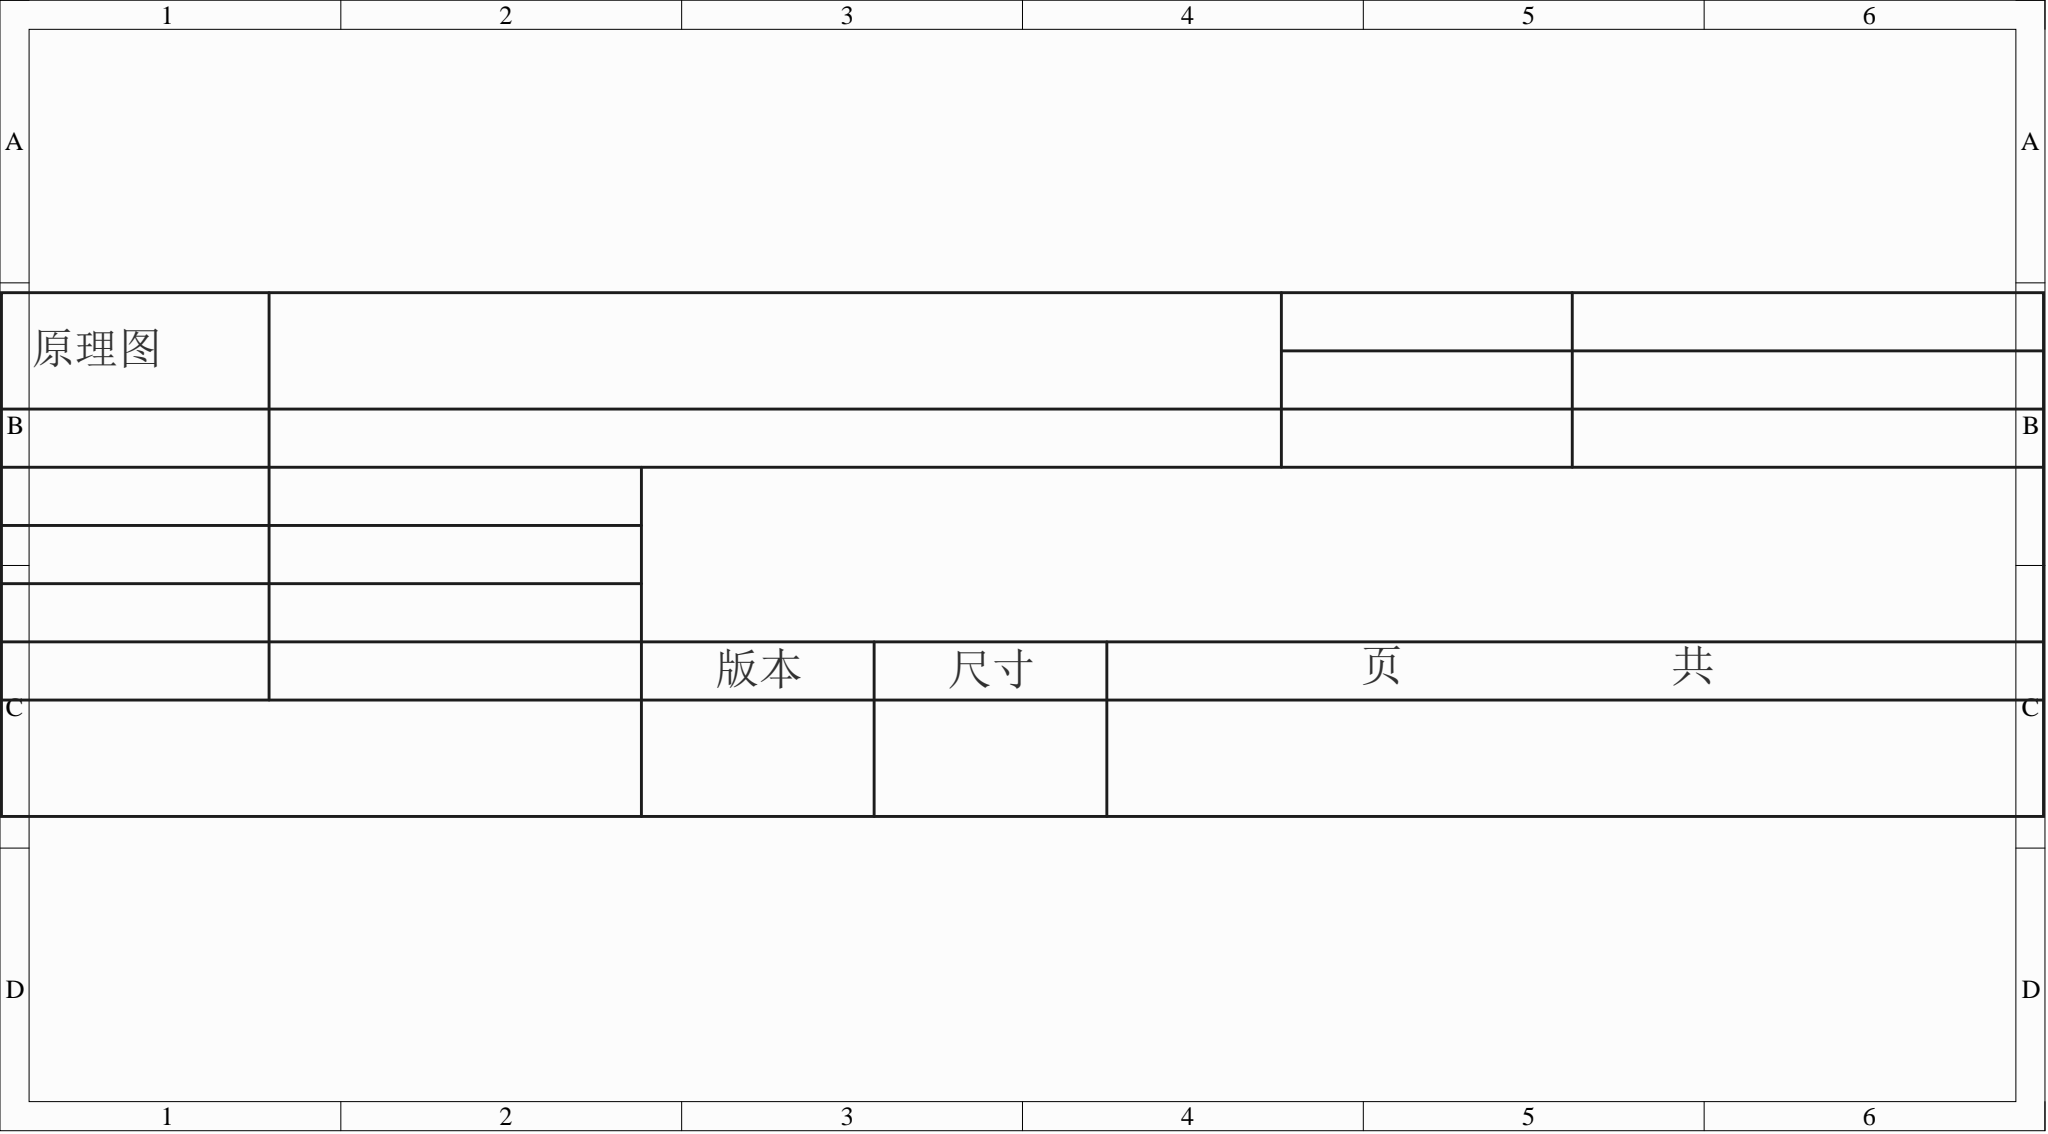Circuit board | Altium Designer | 82 parts | 112 nets
Bill of materials:
Comment,Description,Designator,Footprint,LibRef,Quantity
"","","LED1, LED2, LED3","LED-SEG-TH_10P-L12.6-W19.0-P2.54-S15.24-BL","LED_SEG_TH_0.56x1","3"
"1K","","R1, R2, R3, R4, R5, R6, R7, R8, R9, R10, R11, R12, R13, R14, R15, R16, R17, R18, R19, R20, R21, R22, R23","R0603","Res_0603","23"
"轻触按键3*4*H","","SW1, SW2, SW3, SW4, SW5, SW6, SW7, SW8, SW9, SW10, SW11","SW-SMD_L4.0-W2.9-LS5.0","轻触按键3*4*H","11"
"DSWB04LHGET","","SW12, SW13, SW14","SW-TH_DSWB04LHGET","DSWB04LHGET","3"
"SN74LS04NSR","","U1","SOIC-14_L10.0-W5.5-P1.27-LS7.8-BL","SN74LS04NSR","1"
"SN74LS47NSR","","U2, U5, U10","SO-16_L10.2-W5.3-P1.27-LS7.8-BL","SN74LS47NSR","3"
"SN74LS85NS","","U3, U8, U11","SOIC-16_L10.8-W5.5-P1.27-LS7.8-BL","SN74LS85NS","3"
"SN74HC21NSR","","U6, U7, U14, U15","SO-14_L10.2-W5.3-P1.27-LS7.8-BL-1","SN74HC21NSR","4"
"SN74S175N","","U9, U13, U33","PDIP-16_L19.3-W6.4-P2.54-LS7.9-BL","SN74S175N","3"
"NC7SU04M5-FS","","U16, U24, U28, U30, U35, U52, U53","SOT-23-5_L2.9-W1.6-P0.95-LS2.8-BR","NC7SU04M5-FS","7"
"NC7S08M5","","U19","SOT-23-5_L3.0-W1.5-P0.95-LS2.8-BL","NC7S08M5","1"
"SN74LS147N(LX)","","U20","PDIP-16_L19.3-W6.4-P2.54-LS7.94-BL","SN74LS147N(LX)","1"
"NC7S08M5X","","U25, U26, U31, U36, U37, U39, U40, U41, U42, U58","SOT-23-5_L3.0-W1.7-P0.95-LS2.8-BR","NC7S08M5X","10"
"NC7S02P5X","","U29, U38, U43, U55","SC-70-5_L2.1-W1.3-P0.65-LS2.1-BL","NC7S02P5X","4"
"SN74LS161N(LX)","","U56, U57","PDIP-16_L19.3-W6.4-P2.54-LS7.94-BL","SN74LS161N(LX)","2"
"","","X1, X3, X4","LED_TH-3mm","LED_TH-R_3mm","3"
Netlist (Protel format):
[
LED1
LED-SEG-TH_10P-L12.6-W19.0-P2.54-S15.24-BL




]
[
LED2
LED-SEG-TH_10P-L12.6-W19.0-P2.54-S15.24-BL




]
[
LED3
LED-SEG-TH_10P-L12.6-W19.0-P2.54-S15.24-BL




]
[
R1
R0603
1K



]
[
R2
R0603
1K



]
[
R3
R0603
1K



]
[
R4
R0603
1K



]
[
R5
R0603
1K



]
[
R6
R0603
1K



]
[
R7
R0603
1K



]
[
R8
R0603
1K



]
[
R9
R0603
1K



]
[
R10
R0603
1K



]
[
R11
R0603
1K



]
[
R12
R0603
1K



]
[
R13
R0603
1K



]
[
R14
R0603
1K



]
[
R15
R0603
1K



]
[
R16
R0603
1K



]
[
R17
R0603
1K



]
[
R18
R0603
1K



]
[
R19
R0603
1K



]
[
R20
R0603
1K



]
[
R21
R0603
1K



]
[
R22
R0603
1K



]
[
R23
R0603
1K



]
[
SW1
SW-SMD_L4.0-W2.9-LS5.0
轻触按键3*4*H



]
[
SW2
SW-SMD_L4.0-W2.9-LS5.0
轻触按键3*4*H



]
[
SW3
SW-SMD_L4.0-W2.9-LS5.0
轻触按键3*4*H



]
[
SW4
SW-SMD_L4.0-W2.9-LS5.0
轻触按键3*4*H



]
[
SW5
SW-SMD_L4.0-W2.9-LS5.0
轻触按键3*4*H



]
[
SW6
SW-SMD_L4.0-W2.9-LS5.0
轻触按键3*4*H



]
[
SW7
SW-SMD_L4.0-W2.9-LS5.0
轻触按键3*4*H



]
[
SW8
SW-SMD_L4.0-W2.9-LS5.0
轻触按键3*4*H



]
[
SW9
SW-SMD_L4.0-W2.9-LS5.0
轻触按键3*4*H



]
[
SW10
SW-SMD_L4.0-W2.9-LS5.0
轻触按键3*4*H



]
[
SW11
SW-SMD_L4.0-W2.9-LS5.0
轻触按键3*4*H



]
[
SW12
SW-TH_DSWB04LHGET
DSWB04LHGET



]
[
SW13
SW-TH_DSWB04LHGET
DSWB04LHGET



]
[
SW14
SW-TH_DSWB04LHGET
DSWB04LHGET



]
[
U1
SOIC-14_L10.0-W5.5-P1.27-LS7.8-BL
SN74LS04NSR



]
[
U2
SO-16_L10.2-W5.3-P1.27-LS7.8-BL
SN74LS47NSR



]
[
U3
SOIC-16_L10.8-W5.5-P1.27-LS7.8-BL
SN74LS85NS



]
[
U5
SO-16_L10.2-W5.3-P1.27-LS7.8-BL
SN74LS47NSR



]
[
U6
SO-14_L10.2-W5.3-P1.27-LS7.8-BL-1
SN74HC21NSR



]
[
U7
SO-14_L10.2-W5.3-P1.27-LS7.8-BL-1
SN74HC21NSR



]
[
U8
SOIC-16_L10.8-W5.5-P1.27-LS7.8-BL
SN74LS85NS



]
[
U9
PDIP-16_L19.3-W6.4-P2.54-LS7.9-BL
SN74S175N



]
[
U10
SO-16_L10.2-W5.3-P1.27-LS7.8-BL
SN74LS47NSR



]
[
U11
SOIC-16_L10.8-W5.5-P1.27-LS7.8-BL
SN74LS85NS



]
[
U13
PDIP-16_L19.3-W6.4-P2.54-LS7.9-BL
SN74S175N



]
[
U14
SO-14_L10.2-W5.3-P1.27-LS7.8-BL-1
SN74HC21NSR



]
[
U15
SO-14_L10.2-W5.3-P1.27-LS7.8-BL-1
SN74HC21NSR



]
[
U16
SOT-23-5_L2.9-W1.6-P0.95-LS2.8-BR
NC7SU04M5-FS



]
[
U19
SOT-23-5_L3.0-W1.5-P0.95-LS2.8-BL
NC7S08M5



]
[
U20
PDIP-16_L19.3-W6.4-P2.54-LS7.94-BL
SN74LS147N(LX)



]
[
U24
SOT-23-5_L2.9-W1.6-P0.95-LS2.8-BR
NC7SU04M5-FS



]
[
U25
SOT-23-5_L3.0-W1.7-P0.95-LS2.8-BR
NC7S08M5X



]
[
U26
SOT-23-5_L3.0-W1.7-P0.95-LS2.8-BR
NC7S08M5X



]
[
U28
SOT-23-5_L2.9-W1.6-P0.95-LS2.8-BR
NC7SU04M5-FS



]
[
U29
SC-70-5_L2.1-W1.3-P0.65-LS2.1-BL
NC7S02P5X



]
[
U30
SOT-23-5_L2.9-W1.6-P0.95-LS2.8-BR
NC7SU04M5-FS



]
[
U31
SOT-23-5_L3.0-W1.7-P0.95-LS2.8-BR
NC7S08M5X



]
[
U33
PDIP-16_L19.3-W6.4-P2.54-LS7.9-BL
SN74S175N



]
[
U35
SOT-23-5_L2.9-W1.6-P0.95-LS2.8-BR
NC7SU04M5-FS



]
[
U36
SOT-23-5_L3.0-W1.7-P0.95-LS2.8-BR
NC7S08M5X



]
[
U37
SOT-23-5_L3.0-W1.7-P0.95-LS2.8-BR
NC7S08M5X



]
[
U38
SC-70-5_L2.1-W1.3-P0.65-LS2.1-BL
NC7S02P5X



]
[
U39
SOT-23-5_L3.0-W1.7-P0.95-LS2.8-BR
NC7S08M5X



]
[
U40
SOT-23-5_L3.0-W1.7-P0.95-LS2.8-BR
NC7S08M5X



]
[
U41
SOT-23-5_L3.0-W1.7-P0.95-LS2.8-BR
NC7S08M5X



]
[
U42
SOT-23-5_L3.0-W1.7-P0.95-LS2.8-BR
NC7S08M5X



]
[
U43
SC-70-5_L2.1-W1.3-P0.65-LS2.1-BL
NC7S02P5X



]
[
U52
SOT-23-5_L2.9-W1.6-P0.95-LS2.8-BR
NC7SU04M5-FS



]
[
U53
SOT-23-5_L2.9-W1.6-P0.95-LS2.8-BR
NC7SU04M5-FS



]
[
U55
SC-70-5_L2.1-W1.3-P0.65-LS2.1-BL
NC7S02P5X



]
[
U56
PDIP-16_L19.3-W6.4-P2.54-LS7.94-BL
SN74LS161N(LX)



]
[
U57
PDIP-16_L19.3-W6.4-P2.54-LS7.94-BL
SN74LS161N(LX)



]
[
U58
SOT-23-5_L3.0-W1.7-P0.95-LS2.8-BR
NC7S08M5X



]
[
X1
LED_TH-3mm




]
[
X3
LED_TH-3mm




]
[
X4
LED_TH-3mm




]
(
VCC
LED1-3
LED1-8
LED2-3
LED2-8
LED3-3
LED3-8
R1-2
R2-2
R3-2
R4-2
R5-2
R6-2
R7-2
R8-2
R9-2
R10-2
R11-2
R12-2
R13-2
R14-2
R15-2
R16-2
R17-2
R18-2
R19-2
R20-2
R21-2
R22-2
R23-2
U1-14
U2-3
U2-4
U2-5
U2-16
U3-3
U3-16
U5-3
U5-4
U5-5
U5-16
U6-14
U7-14
U8-3
U8-16
U9-1
U9-16
U10-3
U10-4
U10-5
U10-16
U11-3
U11-16
U13-1
U13-16
U14-14
U15-4
U15-5
U15-14
U16-5
U19-5
U20-16
U24-5
U25-5
U26-5
U28-5
U29-5
U30-5
U31-5
U33-1
U33-16
U35-5
U36-5
U37-5
U38-5
U39-5
U40-5
U41-5
U42-5
U43-5
U52-5
U53-5
U55-5
U56-7
U56-10
U56-16
U57-7
U57-10
U57-16
U58-5
)
(
NetU58_4
U58-4
X4-1
)
(
NetU57_14
U57-14
U58-1
)
(
NetU57_13
U57-13
U58-2
)
(
NetU42_2
U42-2
U43-4
)
(
NetU41_2
U41-2
U42-4
)
(
NetU39_4
U39-4
U53-2
)
(
NetU39_2
U39-2
U40-4
)
(
NetU37_2
U37-2
U38-4
)
(
NetU36_4
U36-4
U52-2
)
(
NetU36_2
U36-2
U37-4
)
(
NetU33_9
U33-9
U35-4
)
(
NetU30_4
U30-4
U31-2
)
(
NetU29_4
U29-4
U31-1
)
(
NetU29_2
U29-2
U37-1
U40-2
U43-2
U55-2
U56-13
)
(
NetU29_1
U29-1
U38-2
U42-1
U55-1
U56-12
)
(
NetU28_2
U28-2
U41-4
U57-2
)
(
NetU26_2
U26-2
U30-2
U38-1
U40-1
U43-1
U56-14
)
(
NetU26_1
U26-1
U55-4
)
(
NetU25_4
U25-4
U35-2
)
(
NetU25_2
U25-2
U26-4
)
(
NetU24_4
U24-4
U56-2
)
(
NetU19_4
U19-4
U56-1
U56-9
)
(
NetU15_6
U15-6
X1-1
)
(
NetU15_2
U15-2
U16-4
U57-1
U57-9
)
(
NetU14_9
U14-9
U15-1
U31-4
)
(
NetU14_8
U14-8
U16-2
X3-1
)
(
NetU13_9
U13-9
U53-4
)
(
NetU11_6
U11-6
U14-10
)
(
NetU10_7
U10-7
U11-9
U13-2
)
(
NetU10_6
U10-6
U11-1
U13-15
)
(
NetU10_2
U10-2
U11-14
U13-10
)
(
NetU10_1
U10-1
U11-11
U13-7
)
(
NetU9_9
U9-9
U52-4
)
(
NetU8_6
U8-6
U14-12
)
(
NetU7_8
U7-8
U24-2
U25-1
U36-1
U39-1
U41-1
)
(
NetU6_8
U6-8
U7-10
)
(
NetU6_6
U6-6
U7-9
)
(
NetU5_7
U5-7
U8-9
U33-2
)
(
NetU5_6
U5-6
U8-1
U33-15
)
(
NetU5_2
U5-2
U8-14
U33-10
)
(
NetU5_1
U5-1
U8-11
U33-7
)
(
NetU3_6
U3-6
U14-13
)
(
NetU2_7
U2-7
U3-9
U9-2
U13-4
)
(
NetU2_6
U2-6
U3-1
U9-15
U13-13
)
(
NetU2_2
U2-2
U3-14
U9-10
U13-12
)
(
NetU2_1
U2-1
U3-11
U9-7
U13-5
)
(
NetU1_9
U1-9
U20-14
)
(
NetU1_8
U1-8
U9-13
U33-13
)
(
NetU1_6
U1-6
U9-12
U33-12
)
(
NetU1_5
U1-5
U20-6
)
(
NetU1_4
U1-4
U9-5
U33-5
)
(
NetU1_3
U1-3
U20-7
)
(
NetU1_2
U1-2
U9-4
U33-4
)
(
NetU1_1
U1-1
U20-9
)
(
NetSW14_8
SW14-8
U11-15
)
(
NetSW14_7
SW14-7
U11-13
)
(
NetSW14_6
SW14-6
U11-12
)
(
NetSW14_5
SW14-5
U11-10
)
(
NetSW13_8
SW13-8
U3-15
)
(
NetSW13_7
SW13-7
U3-13
)
(
NetSW13_6
SW13-6
U3-12
)
(
NetSW13_5
SW13-5
U3-10
)
(
NetSW12_8
SW12-8
U8-15
)
(
NetSW12_7
SW12-7
U8-13
)
(
NetSW12_6
SW12-6
U8-12
)
(
NetSW12_5
SW12-5
U8-10
)
(
NetR23_1
R23-1
SW14-4
)
(
NetR22_1
R22-1
SW14-3
)
(
NetR21_1
R21-1
SW14-2
)
(
NetR20_1
R20-1
SW14-1
)
(
NetR19_1
R19-1
SW13-4
)
(
NetR18_1
R18-1
SW13-3
)
(
NetR17_1
R17-1
SW13-2
)
(
NetR16_1
R16-1
SW13-1
)
(
NetR15_1
R15-1
SW12-4
)
(
NetR14_1
R14-1
SW12-3
)
(
NetR13_1
R13-1
SW12-2
)
(
NetR12_1
R12-1
SW12-1
)
(
NetR11_1
R11-1
SW11-1
U19-1
)
(
NetR10_1
R10-1
SW10-2
U7-12
U20-10
)
(
NetR9_1
R9-1
SW9-2
U6-10
U20-3
)
(
NetR8_1
R8-1
SW8-2
U6-4
U20-13
)
(
NetR7_1
R7-1
SW7-2
U7-13
)
(
NetR6_1
R6-1
SW6-2
U6-13
U20-5
)
(
NetR5_1
R5-1
SW5-2
U6-9
U20-2
)
(
NetR4_1
R4-1
SW4-2
U6-2
U20-12
)
(
NetR3_1
R3-1
SW3-2
U6-12
U20-4
)
(
NetR2_1
R2-1
SW2-2
U6-5
U20-1
)
(
NetR1_1
R1-1
SW1-2
U6-1
U20-11
)
(
NetLED3_10
LED3-10
U10-14
)
(
NetLED3_9
LED3-9
U10-15
)
(
NetLED3_7
LED3-7
U10-13
)
(
NetLED3_6
LED3-6
U10-12
)
(
NetLED3_4
LED3-4
U10-11
)
(
NetLED3_2
LED3-2
U10-10
)
(
NetLED3_1
LED3-1
U10-9
)
(
NetLED2_10
LED2-10
U2-14
)
(
NetLED2_9
LED2-9
U2-15
)
(
NetLED2_7
LED2-7
U2-13
)
(
NetLED2_6
LED2-6
U2-12
)
(
NetLED2_4
LED2-4
U2-11
)
(
NetLED2_2
LED2-2
U2-10
)
(
NetLED2_1
LED2-1
U2-9
)
(
NetLED1_10
LED1-10
U5-14
)
(
NetLED1_9
LED1-9
U5-15
)
(
NetLED1_7
LED1-7
U5-13
)
(
NetLED1_6
LED1-6
U5-12
)
(
NetLED1_4
LED1-4
U5-11
)
(
NetLED1_2
LED1-2
U5-10
)
(
NetLED1_1
LED1-1
U5-9
)
(
GND
SW1-1
SW2-1
SW3-1
SW4-1
SW5-1
SW6-1
SW7-1
SW8-1
SW9-1
SW10-1
SW11-2
U1-7
U2-8
U3-8
U5-8
U6-7
U7-7
U8-8
U9-8
U10-8
U11-8
U13-8
U14-7
U15-7
U16-3
U19-2
U19-3
U20-8
U24-3
U25-3
U26-3
U28-3
U28-4
U29-3
U30-3
U31-3
U33-8
U35-3
U36-3
U37-3
U38-3
U39-3
U40-3
U41-3
U42-3
U43-3
U52-3
U53-3
U55-3
U56-3
U56-4
U56-5
U56-6
U56-8
U57-3
U57-4
U57-5
U57-6
U57-8
U58-3
X1-2
X3-2
X4-2
)